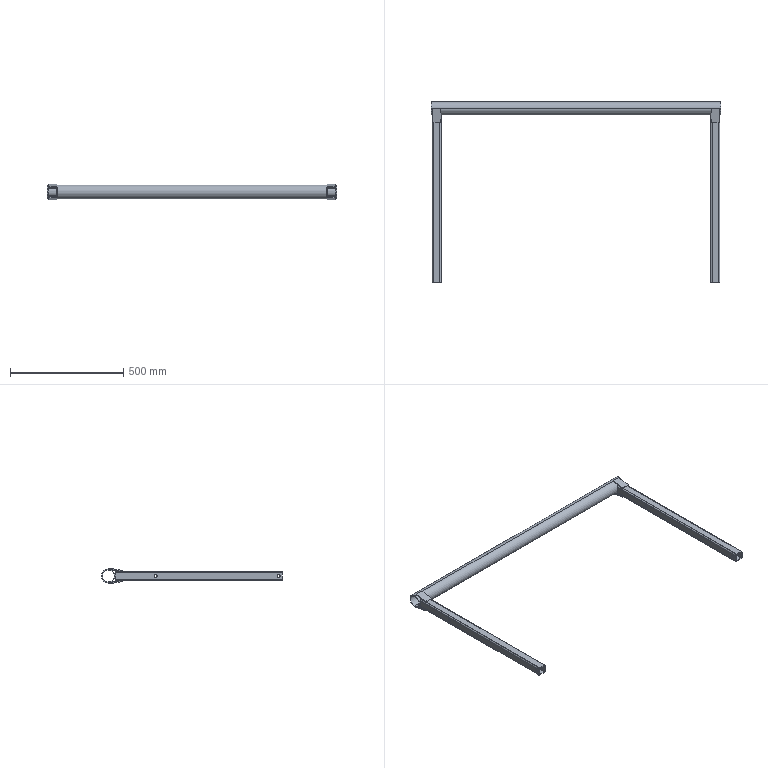Part | SolidWorks | features 3DProfileFeature 2, HoleWzd 2, ICE 2, MirrorSolid 2, WeldMemberFeat 2, WeldmentFeature 1 | 7 solids | 82 faces | box 1280 x 800 x 70.292 mm | volume 1562390 mm3 | plane 46 | cylinder 36 | commonest cylinder face diameters 13 x16 6 x8 12 x8 52 x2 60 x2